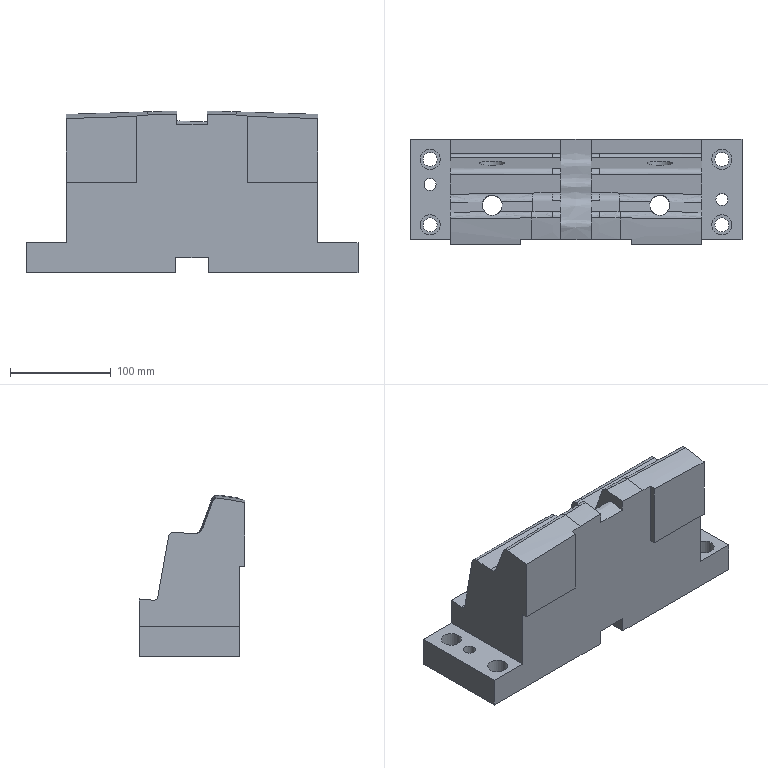Part | NX | features solid 2 | 1 solid | 82 faces | box 330 x 105 x 161.017 mm | volume 3009962 mm3 | spline 37 | plane 27 | cylinder 18 | commonest cylinder face diameters 20 x6 14 x4 4 x2 12 x2 18.6 x2 25 x2